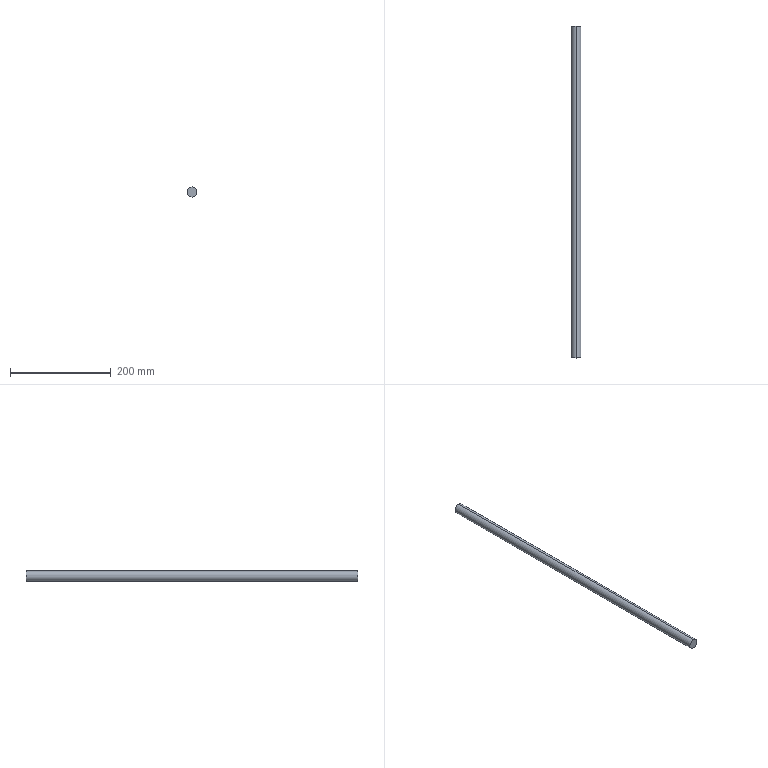Part | SolidWorks | features Extrusion 1 | 1 solid | 4 faces | box 20 x 660 x 20 mm | volume 207345 mm3 | cylinder 2 | plane 2 | commonest cylinder face diameters 20 x2
STEP:
#1=CARTESIAN_POINT('',(0.,660.,10.));
#2=VERTEX_POINT('',#1);
#3=CARTESIAN_POINT('',(0.,660.,-10.));
#4=VERTEX_POINT('',#3);
#5=CARTESIAN_POINT('',(0.,660.,0.));
#6=DIRECTION('',(0.,1.,0.));
#7=DIRECTION('',(0.,0.,1.));
#8=AXIS2_PLACEMENT_3D('',#5,#6,#7);
#9=CIRCLE('',#8,10.);
#10=EDGE_CURVE('',#2,#4,#9,.T.);
#11=ORIENTED_EDGE('',*,*,#10,.F.);
#12=CARTESIAN_POINT('',(0.,0.,10.));
#13=VERTEX_POINT('',#12);
#14=CARTESIAN_POINT('',(0.,660.,10.));
#15=DIRECTION('',(0.,-1.,0.));
#16=VECTOR('',#15,1000.);
#17=LINE('',#14,#16);
#18=EDGE_CURVE('',#2,#13,#17,.T.);
#19=ORIENTED_EDGE('',*,*,#18,.T.);
#20=CARTESIAN_POINT('',(0.,0.,-10.));
#21=VERTEX_POINT('',#20);
#22=CARTESIAN_POINT('',(0.,0.,0.));
#23=DIRECTION('',(0.,1.,0.));
#24=DIRECTION('',(0.,0.,1.));
#25=AXIS2_PLACEMENT_3D('',#22,#23,#24);
#26=CIRCLE('',#25,10.);
#27=EDGE_CURVE('',#13,#21,#26,.T.);
#28=ORIENTED_EDGE('',*,*,#27,.T.);
#29=CARTESIAN_POINT('',(0.,660.,-10.));
#30=DIRECTION('',(0.,-1.,0.));
#31=VECTOR('',#30,1000.);
#32=LINE('',#29,#31);
#33=EDGE_CURVE('',#4,#21,#32,.T.);
#34=ORIENTED_EDGE('',*,*,#33,.F.);
#35=EDGE_LOOP('',(#11,#19,#28,#34));
#36=FACE_OUTER_BOUND('',#35,.T.);
#37=CARTESIAN_POINT('',(0.,660.,0.));
#38=DIRECTION('',(0.,-1.,0.));
#39=DIRECTION('',(0.,0.,-1.));
#40=AXIS2_PLACEMENT_3D('',#37,#38,#39);
#41=CYLINDRICAL_SURFACE('',#40,10.);
#42=ADVANCED_FACE('',(#36),#41,.T.);
#43=ORIENTED_EDGE('',*,*,#18,.F.);
#44=CARTESIAN_POINT('',(0.,660.,0.));
#45=DIRECTION('',(0.,1.,0.));
#46=DIRECTION('',(0.,0.,1.));
#47=AXIS2_PLACEMENT_3D('',#44,#45,#46);
#48=CIRCLE('',#47,10.);
#49=EDGE_CURVE('',#4,#2,#48,.T.);
#50=ORIENTED_EDGE('',*,*,#49,.F.);
#51=ORIENTED_EDGE('',*,*,#33,.T.);
#52=CARTESIAN_POINT('',(0.,0.,0.));
#53=DIRECTION('',(0.,1.,0.));
#54=DIRECTION('',(0.,0.,1.));
#55=AXIS2_PLACEMENT_3D('',#52,#53,#54);
#56=CIRCLE('',#55,10.);
#57=EDGE_CURVE('',#21,#13,#56,.T.);
#58=ORIENTED_EDGE('',*,*,#57,.T.);
#59=EDGE_LOOP('',(#43,#50,#51,#58));
#60=FACE_OUTER_BOUND('',#59,.T.);
#61=CARTESIAN_POINT('',(0.,660.,0.));
#62=DIRECTION('',(0.,-1.,0.));
#63=DIRECTION('',(0.,0.,-1.));
#64=AXIS2_PLACEMENT_3D('',#61,#62,#63);
#65=CYLINDRICAL_SURFACE('',#64,10.);
#66=ADVANCED_FACE('',(#60),#65,.T.);
#67=ORIENTED_EDGE('',*,*,#49,.T.);
#68=ORIENTED_EDGE('',*,*,#10,.T.);
#69=EDGE_LOOP('',(#67,#68));
#70=FACE_OUTER_BOUND('',#69,.T.);
#71=CARTESIAN_POINT('',(0.,660.,0.));
#72=DIRECTION('',(0.,1.,0.));
#73=DIRECTION('',(0.,0.,1.));
#74=AXIS2_PLACEMENT_3D('',#71,#72,#73);
#75=PLANE('',#74);
#76=ADVANCED_FACE('',(#70),#75,.T.);
#77=ORIENTED_EDGE('',*,*,#57,.F.);
#78=ORIENTED_EDGE('',*,*,#27,.F.);
#79=EDGE_LOOP('',(#77,#78));
#80=FACE_OUTER_BOUND('',#79,.T.);
#81=CARTESIAN_POINT('',(0.,0.,0.));
#82=DIRECTION('',(0.,1.,0.));
#83=DIRECTION('',(0.,0.,1.));
#84=AXIS2_PLACEMENT_3D('',#81,#82,#83);
#85=PLANE('',#84);
#86=ADVANCED_FACE('',(#80),#85,.F.);
#87=CLOSED_SHELL('',(#42,#66,#76,#86));
#88=MANIFOLD_SOLID_BREP('',#87);
#89=CARTESIAN_POINT('',(0.,0.,0.));
#90=DIRECTION('',(0.,0.,1.));
#91=DIRECTION('',(1.,0.,0.));
#92=AXIS2_PLACEMENT_3D('',#89,#90,#91);
#93=(LENGTH_UNIT()NAMED_UNIT(*)SI_UNIT(.MILLI.,.METRE.));
#94=UNCERTAINTY_MEASURE_WITH_UNIT(LENGTH_MEASURE(0.00001),#93,'','');
#95=(NAMED_UNIT(*)PLANE_ANGLE_UNIT()SI_UNIT($,.RADIAN.));
#96=(NAMED_UNIT(*)SI_UNIT($,.STERADIAN.)SOLID_ANGLE_UNIT());
#97=(GEOMETRIC_REPRESENTATION_CONTEXT(3)GLOBAL_UNCERTAINTY_ASSIGNED_CONTEXT((#94))GLOBAL_UNIT_ASSIGNED_CONTEXT((#93,#95,#96))REPRESENTATION_CONTEXT('',''));
#98=ADVANCED_BREP_SHAPE_REPRESENTATION('',(#88,#92),#97);